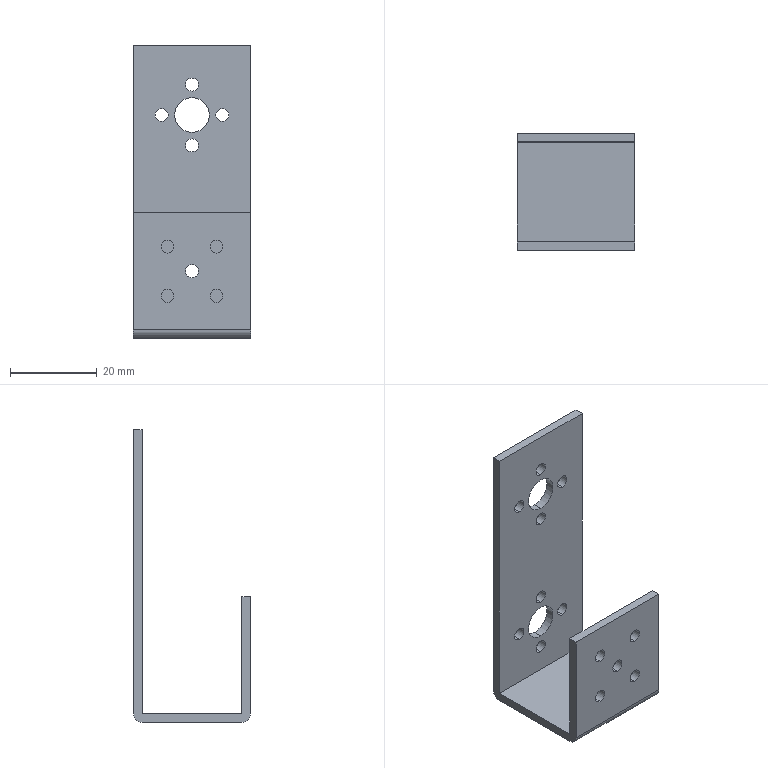Part | SolidWorks | features ICE 5, Extrusion 1, Fillet 1 | 1 solid | 42 faces | box 27 x 27 x 67.5 mm | volume 6022 mm3 | cylinder 32 | plane 10 | commonest cylinder face diameters 3 x26 8 x4 4 x2
STEP:
#1=CARTESIAN_POINT('',(0.,11.5,46.));
#2=VERTEX_POINT('',#1);
#3=CARTESIAN_POINT('',(0.,11.5,43.));
#4=VERTEX_POINT('',#3);
#5=CARTESIAN_POINT('',(0.,11.5,44.5));
#6=DIRECTION('',(0.,-1.,0.));
#7=DIRECTION('',(-1.,0.,0.));
#8=AXIS2_PLACEMENT_3D('',#5,#6,#7);
#9=CIRCLE('',#8,1.5);
#10=EDGE_CURVE('',#2,#4,#9,.T.);
#11=ORIENTED_EDGE('',*,*,#10,.T.);
#12=CARTESIAN_POINT('',(0.,13.5,43.));
#13=VERTEX_POINT('',#12);
#14=CARTESIAN_POINT('',(0.,0.1863,43.));
#15=DIRECTION('',(0.,1.,0.));
#16=VECTOR('',#15,1000.);
#17=LINE('',#14,#16);
#18=EDGE_CURVE('',#4,#13,#17,.T.);
#19=ORIENTED_EDGE('',*,*,#18,.T.);
#20=CARTESIAN_POINT('',(0.,13.5,46.));
#21=VERTEX_POINT('',#20);
#22=CARTESIAN_POINT('',(0.,13.5,44.5));
#23=DIRECTION('',(0.,1.,0.));
#24=DIRECTION('',(0.,0.,1.));
#25=AXIS2_PLACEMENT_3D('',#22,#23,#24);
#26=CIRCLE('',#25,1.5);
#27=EDGE_CURVE('',#13,#21,#26,.T.);
#28=ORIENTED_EDGE('',*,*,#27,.T.);
#29=CARTESIAN_POINT('',(0.,0.1863,46.));
#30=DIRECTION('',(0.,1.,0.));
#31=VECTOR('',#30,1000.);
#32=LINE('',#29,#31);
#33=EDGE_CURVE('',#2,#21,#32,.T.);
#34=ORIENTED_EDGE('',*,*,#33,.F.);
#35=EDGE_LOOP('',(#11,#19,#28,#34));
#36=FACE_OUTER_BOUND('',#35,.T.);
#37=CARTESIAN_POINT('',(0.,0.1863,44.5));
#38=DIRECTION('',(0.,1.,0.));
#39=DIRECTION('',(0.,0.,1.));
#40=AXIS2_PLACEMENT_3D('',#37,#38,#39);
#41=CYLINDRICAL_SURFACE('',#40,1.5);
#42=ADVANCED_FACE('',(#36),#41,.F.);
#43=CARTESIAN_POINT('',(7.,11.5,53.));
#44=VERTEX_POINT('',#43);
#45=CARTESIAN_POINT('',(7.,11.5,50.));
#46=VERTEX_POINT('',#45);
#47=CARTESIAN_POINT('',(7.,11.5,51.5));
#48=DIRECTION('',(0.,-1.,0.));
#49=DIRECTION('',(-1.,0.,0.));
#50=AXIS2_PLACEMENT_3D('',#47,#48,#49);
#51=CIRCLE('',#50,1.5);
#52=EDGE_CURVE('',#44,#46,#51,.T.);
#53=ORIENTED_EDGE('',*,*,#52,.T.);
#54=CARTESIAN_POINT('',(7.,13.5,50.));
#55=VERTEX_POINT('',#54);
#56=CARTESIAN_POINT('',(7.,0.1863,50.));
#57=DIRECTION('',(0.,1.,0.));
#58=VECTOR('',#57,1000.);
#59=LINE('',#56,#58);
#60=EDGE_CURVE('',#46,#55,#59,.T.);
#61=ORIENTED_EDGE('',*,*,#60,.T.);
#62=CARTESIAN_POINT('',(7.,13.5,53.));
#63=VERTEX_POINT('',#62);
#64=CARTESIAN_POINT('',(7.,13.5,51.5));
#65=DIRECTION('',(0.,1.,0.));
#66=DIRECTION('',(0.,0.,1.));
#67=AXIS2_PLACEMENT_3D('',#64,#65,#66);
#68=CIRCLE('',#67,1.5);
#69=EDGE_CURVE('',#55,#63,#68,.T.);
#70=ORIENTED_EDGE('',*,*,#69,.T.);
#71=CARTESIAN_POINT('',(7.,0.1863,53.));
#72=DIRECTION('',(0.,1.,0.));
#73=VECTOR('',#72,1000.);
#74=LINE('',#71,#73);
#75=EDGE_CURVE('',#44,#63,#74,.T.);
#76=ORIENTED_EDGE('',*,*,#75,.F.);
#77=EDGE_LOOP('',(#53,#61,#70,#76));
#78=FACE_OUTER_BOUND('',#77,.T.);
#79=CARTESIAN_POINT('',(7.,0.1863,51.5));
#80=DIRECTION('',(0.,1.,0.));
#81=DIRECTION('',(0.,0.,1.));
#82=AXIS2_PLACEMENT_3D('',#79,#80,#81);
#83=CYLINDRICAL_SURFACE('',#82,1.5);
#84=ADVANCED_FACE('',(#78),#83,.F.);
#85=CARTESIAN_POINT('',(0.,11.5,60.));
#86=VERTEX_POINT('',#85);
#87=CARTESIAN_POINT('',(0.,11.5,57.));
#88=VERTEX_POINT('',#87);
#89=CARTESIAN_POINT('',(0.,11.5,58.5));
#90=DIRECTION('',(0.,-1.,0.));
#91=DIRECTION('',(-1.,0.,0.));
#92=AXIS2_PLACEMENT_3D('',#89,#90,#91);
#93=CIRCLE('',#92,1.5);
#94=EDGE_CURVE('',#86,#88,#93,.T.);
#95=ORIENTED_EDGE('',*,*,#94,.T.);
#96=CARTESIAN_POINT('',(0.,13.5,57.));
#97=VERTEX_POINT('',#96);
#98=CARTESIAN_POINT('',(0.,0.1863,57.));
#99=DIRECTION('',(0.,1.,0.));
#100=VECTOR('',#99,1000.);
#101=LINE('',#98,#100);
#102=EDGE_CURVE('',#88,#97,#101,.T.);
#103=ORIENTED_EDGE('',*,*,#102,.T.);
#104=CARTESIAN_POINT('',(0.,13.5,60.));
#105=VERTEX_POINT('',#104);
#106=CARTESIAN_POINT('',(0.,13.5,58.5));
#107=DIRECTION('',(0.,1.,0.));
#108=DIRECTION('',(0.,0.,1.));
#109=AXIS2_PLACEMENT_3D('',#106,#107,#108);
#110=CIRCLE('',#109,1.5);
#111=EDGE_CURVE('',#97,#105,#110,.T.);
#112=ORIENTED_EDGE('',*,*,#111,.T.);
#113=CARTESIAN_POINT('',(0.,0.1863,60.));
#114=DIRECTION('',(0.,1.,0.));
#115=VECTOR('',#114,1000.);
#116=LINE('',#113,#115);
#117=EDGE_CURVE('',#86,#105,#116,.T.);
#118=ORIENTED_EDGE('',*,*,#117,.F.);
#119=EDGE_LOOP('',(#95,#103,#112,#118));
#120=FACE_OUTER_BOUND('',#119,.T.);
#121=CARTESIAN_POINT('',(0.,0.1863,58.5));
#122=DIRECTION('',(0.,1.,0.));
#123=DIRECTION('',(0.,0.,1.));
#124=AXIS2_PLACEMENT_3D('',#121,#122,#123);
#125=CYLINDRICAL_SURFACE('',#124,1.5);
#126=ADVANCED_FACE('',(#120),#125,.F.);
#127=CARTESIAN_POINT('',(-7.,11.5,53.));
#128=VERTEX_POINT('',#127);
#129=CARTESIAN_POINT('',(-7.,11.5,50.));
#130=VERTEX_POINT('',#129);
#131=CARTESIAN_POINT('',(-7.,11.5,51.5));
#132=DIRECTION('',(0.,-1.,0.));
#133=DIRECTION('',(-1.,0.,0.));
#134=AXIS2_PLACEMENT_3D('',#131,#132,#133);
#135=CIRCLE('',#134,1.5);
#136=EDGE_CURVE('',#128,#130,#135,.T.);
#137=ORIENTED_EDGE('',*,*,#136,.T.);
#138=CARTESIAN_POINT('',(-7.,13.5,50.));
#139=VERTEX_POINT('',#138);
#140=CARTESIAN_POINT('',(-7.,0.1863,50.));
#141=DIRECTION('',(0.,1.,0.));
#142=VECTOR('',#141,1000.);
#143=LINE('',#140,#142);
#144=EDGE_CURVE('',#130,#139,#143,.T.);
#145=ORIENTED_EDGE('',*,*,#144,.T.);
#146=CARTESIAN_POINT('',(-7.,13.5,53.));
#147=VERTEX_POINT('',#146);
#148=CARTESIAN_POINT('',(-7.,13.5,51.5));
#149=DIRECTION('',(0.,1.,0.));
#150=DIRECTION('',(0.,0.,1.));
#151=AXIS2_PLACEMENT_3D('',#148,#149,#150);
#152=CIRCLE('',#151,1.5);
#153=EDGE_CURVE('',#139,#147,#152,.T.);
#154=ORIENTED_EDGE('',*,*,#153,.T.);
#155=CARTESIAN_POINT('',(-7.,0.1863,53.));
#156=DIRECTION('',(0.,1.,0.));
#157=VECTOR('',#156,1000.);
#158=LINE('',#155,#157);
#159=EDGE_CURVE('',#128,#147,#158,.T.);
#160=ORIENTED_EDGE('',*,*,#159,.F.);
#161=EDGE_LOOP('',(#137,#145,#154,#160));
#162=FACE_OUTER_BOUND('',#161,.T.);
#163=CARTESIAN_POINT('',(-7.,0.1863,51.5));
#164=DIRECTION('',(0.,1.,0.));
#165=DIRECTION('',(0.,0.,1.));
#166=AXIS2_PLACEMENT_3D('',#163,#164,#165);
#167=CYLINDRICAL_SURFACE('',#166,1.5);
#168=ADVANCED_FACE('',(#162),#167,.F.);
#169=CARTESIAN_POINT('',(0.,11.5,55.5));
#170=VERTEX_POINT('',#169);
#171=CARTESIAN_POINT('',(0.,11.5,47.5));
#172=VERTEX_POINT('',#171);
#173=CARTESIAN_POINT('',(0.,11.5,51.5));
#174=DIRECTION('',(0.,-1.,0.));
#175=DIRECTION('',(-1.,0.,0.));
#176=AXIS2_PLACEMENT_3D('',#173,#174,#175);
#177=CIRCLE('',#176,4.);
#178=EDGE_CURVE('',#170,#172,#177,.T.);
#179=ORIENTED_EDGE('',*,*,#178,.T.);
#180=CARTESIAN_POINT('',(0.,13.5,47.5));
#181=VERTEX_POINT('',#180);
#182=CARTESIAN_POINT('',(0.,0.1863,47.5));
#183=DIRECTION('',(0.,1.,0.));
#184=VECTOR('',#183,1000.);
#185=LINE('',#182,#184);
#186=EDGE_CURVE('',#172,#181,#185,.T.);
#187=ORIENTED_EDGE('',*,*,#186,.T.);
#188=CARTESIAN_POINT('',(0.,13.5,55.5));
#189=VERTEX_POINT('',#188);
#190=CARTESIAN_POINT('',(0.,13.5,51.5));
#191=DIRECTION('',(0.,1.,0.));
#192=DIRECTION('',(0.,0.,1.));
#193=AXIS2_PLACEMENT_3D('',#190,#191,#192);
#194=CIRCLE('',#193,4.);
#195=EDGE_CURVE('',#181,#189,#194,.T.);
#196=ORIENTED_EDGE('',*,*,#195,.T.);
#197=CARTESIAN_POINT('',(0.,0.1863,55.5));
#198=DIRECTION('',(0.,1.,0.));
#199=VECTOR('',#198,1000.);
#200=LINE('',#197,#199);
#201=EDGE_CURVE('',#170,#189,#200,.T.);
#202=ORIENTED_EDGE('',*,*,#201,.F.);
#203=EDGE_LOOP('',(#179,#187,#196,#202));
#204=FACE_OUTER_BOUND('',#203,.T.);
#205=CARTESIAN_POINT('',(0.,0.1863,51.5));
#206=DIRECTION('',(0.,1.,0.));
#207=DIRECTION('',(0.,0.,1.));
#208=AXIS2_PLACEMENT_3D('',#205,#206,#207);
#209=CYLINDRICAL_SURFACE('',#208,4.);
#210=ADVANCED_FACE('',(#204),#209,.F.);
#211=CARTESIAN_POINT('',(-5.657,-11.5,8.343));
#212=VERTEX_POINT('',#211);
#213=CARTESIAN_POINT('',(-5.657,-11.5,11.343));
#214=VERTEX_POINT('',#213);
#215=CARTESIAN_POINT('',(-5.657,-11.5,9.843));
#216=DIRECTION('',(0.,1.,0.));
#217=DIRECTION('',(1.,0.,0.));
#218=AXIS2_PLACEMENT_3D('',#215,#216,#217);
#219=CIRCLE('',#218,1.5);
#220=EDGE_CURVE('',#212,#214,#219,.T.);
#221=ORIENTED_EDGE('',*,*,#220,.T.);
#222=CARTESIAN_POINT('',(-5.657,-13.5,11.343));
#223=VERTEX_POINT('',#222);
#224=CARTESIAN_POINT('',(-5.657,13.501,11.343));
#225=DIRECTION('',(0.,-1.,0.));
#226=VECTOR('',#225,1000.);
#227=LINE('',#224,#226);
#228=EDGE_CURVE('',#214,#223,#227,.T.);
#229=ORIENTED_EDGE('',*,*,#228,.T.);
#230=CARTESIAN_POINT('',(-5.657,-13.5,8.343));
#231=VERTEX_POINT('',#230);
#232=CARTESIAN_POINT('',(-5.657,-13.5,9.843));
#233=DIRECTION('',(0.,-1.,0.));
#234=DIRECTION('',(0.,0.,-1.));
#235=AXIS2_PLACEMENT_3D('',#232,#233,#234);
#236=CIRCLE('',#235,1.5);
#237=EDGE_CURVE('',#223,#231,#236,.T.);
#238=ORIENTED_EDGE('',*,*,#237,.T.);
#239=CARTESIAN_POINT('',(-5.657,13.501,8.343));
#240=DIRECTION('',(0.,-1.,0.));
#241=VECTOR('',#240,1000.);
#242=LINE('',#239,#241);
#243=EDGE_CURVE('',#212,#231,#242,.T.);
#244=ORIENTED_EDGE('',*,*,#243,.F.);
#245=EDGE_LOOP('',(#221,#229,#238,#244));
#246=FACE_OUTER_BOUND('',#245,.T.);
#247=CARTESIAN_POINT('',(-5.657,13.501,9.843));
#248=DIRECTION('',(0.,-1.,0.));
#249=DIRECTION('',(0.,0.,-1.));
#250=AXIS2_PLACEMENT_3D('',#247,#248,#249);
#251=CYLINDRICAL_SURFACE('',#250,1.5);
#252=ADVANCED_FACE('',(#246),#251,.F.);
#253=CARTESIAN_POINT('',(5.657,-11.5,8.343));
#254=VERTEX_POINT('',#253);
#255=CARTESIAN_POINT('',(5.657,-11.5,11.343));
#256=VERTEX_POINT('',#255);
#257=CARTESIAN_POINT('',(5.657,-11.5,9.843));
#258=DIRECTION('',(0.,1.,0.));
#259=DIRECTION('',(1.,0.,0.));
#260=AXIS2_PLACEMENT_3D('',#257,#258,#259);
#261=CIRCLE('',#260,1.5);
#262=EDGE_CURVE('',#254,#256,#261,.T.);
#263=ORIENTED_EDGE('',*,*,#262,.T.);
#264=CARTESIAN_POINT('',(5.657,-13.5,11.343));
#265=VERTEX_POINT('',#264);
#266=CARTESIAN_POINT('',(5.657,13.501,11.343));
#267=DIRECTION('',(0.,-1.,0.));
#268=VECTOR('',#267,1000.);
#269=LINE('',#266,#268);
#270=EDGE_CURVE('',#256,#265,#269,.T.);
#271=ORIENTED_EDGE('',*,*,#270,.T.);
#272=CARTESIAN_POINT('',(5.657,-13.5,8.343));
#273=VERTEX_POINT('',#272);
#274=CARTESIAN_POINT('',(5.657,-13.5,9.843));
#275=DIRECTION('',(0.,-1.,0.));
#276=DIRECTION('',(0.,0.,-1.));
#277=AXIS2_PLACEMENT_3D('',#274,#275,#276);
#278=CIRCLE('',#277,1.5);
#279=EDGE_CURVE('',#265,#273,#278,.T.);
#280=ORIENTED_EDGE('',*,*,#279,.T.);
#281=CARTESIAN_POINT('',(5.657,13.501,8.343));
#282=DIRECTION('',(0.,-1.,0.));
#283=VECTOR('',#282,1000.);
#284=LINE('',#281,#283);
#285=EDGE_CURVE('',#254,#273,#284,.T.);
#286=ORIENTED_EDGE('',*,*,#285,.F.);
#287=EDGE_LOOP('',(#263,#271,#280,#286));
#288=FACE_OUTER_BOUND('',#287,.T.);
#289=CARTESIAN_POINT('',(5.657,13.501,9.843));
#290=DIRECTION('',(0.,-1.,0.));
#291=DIRECTION('',(0.,0.,-1.));
#292=AXIS2_PLACEMENT_3D('',#289,#290,#291);
#293=CYLINDRICAL_SURFACE('',#292,1.5);
#294=ADVANCED_FACE('',(#288),#293,.F.);
#295=CARTESIAN_POINT('',(5.657,-11.5,19.657));
#296=VERTEX_POINT('',#295);
#297=CARTESIAN_POINT('',(5.657,-11.5,22.657));
#298=VERTEX_POINT('',#297);
#299=CARTESIAN_POINT('',(5.657,-11.5,21.157));
#300=DIRECTION('',(0.,1.,0.));
#301=DIRECTION('',(1.,0.,0.));
#302=AXIS2_PLACEMENT_3D('',#299,#300,#301);
#303=CIRCLE('',#302,1.5);
#304=EDGE_CURVE('',#296,#298,#303,.T.);
#305=ORIENTED_EDGE('',*,*,#304,.T.);
#306=CARTESIAN_POINT('',(5.657,-13.5,22.657));
#307=VERTEX_POINT('',#306);
#308=CARTESIAN_POINT('',(5.657,13.501,22.657));
#309=DIRECTION('',(0.,-1.,0.));
#310=VECTOR('',#309,1000.);
#311=LINE('',#308,#310);
#312=EDGE_CURVE('',#298,#307,#311,.T.);
#313=ORIENTED_EDGE('',*,*,#312,.T.);
#314=CARTESIAN_POINT('',(5.657,-13.5,19.657));
#315=VERTEX_POINT('',#314);
#316=CARTESIAN_POINT('',(5.657,-13.5,21.157));
#317=DIRECTION('',(0.,-1.,0.));
#318=DIRECTION('',(0.,0.,-1.));
#319=AXIS2_PLACEMENT_3D('',#316,#317,#318);
#320=CIRCLE('',#319,1.5);
#321=EDGE_CURVE('',#307,#315,#320,.T.);
#322=ORIENTED_EDGE('',*,*,#321,.T.);
#323=CARTESIAN_POINT('',(5.657,13.501,19.657));
#324=DIRECTION('',(0.,-1.,0.));
#325=VECTOR('',#324,1000.);
#326=LINE('',#323,#325);
#327=EDGE_CURVE('',#296,#315,#326,.T.);
#328=ORIENTED_EDGE('',*,*,#327,.F.);
#329=EDGE_LOOP('',(#305,#313,#322,#328));
#330=FACE_OUTER_BOUND('',#329,.T.);
#331=CARTESIAN_POINT('',(5.657,13.501,21.157));
#332=DIRECTION('',(0.,-1.,0.));
#333=DIRECTION('',(0.,0.,-1.));
#334=AXIS2_PLACEMENT_3D('',#331,#332,#333);
#335=CYLINDRICAL_SURFACE('',#334,1.5);
#336=ADVANCED_FACE('',(#330),#335,.F.);
#337=CARTESIAN_POINT('',(-5.657,-11.5,19.657));
#338=VERTEX_POINT('',#337);
#339=CARTESIAN_POINT('',(-5.657,-11.5,22.657));
#340=VERTEX_POINT('',#339);
#341=CARTESIAN_POINT('',(-5.657,-11.5,21.157));
#342=DIRECTION('',(0.,1.,0.));
#343=DIRECTION('',(1.,0.,0.));
#344=AXIS2_PLACEMENT_3D('',#341,#342,#343);
#345=CIRCLE('',#344,1.5);
#346=EDGE_CURVE('',#338,#340,#345,.T.);
#347=ORIENTED_EDGE('',*,*,#346,.T.);
#348=CARTESIAN_POINT('',(-5.657,-13.5,22.657));
#349=VERTEX_POINT('',#348);
#350=CARTESIAN_POINT('',(-5.657,13.501,22.657));
#351=DIRECTION('',(0.,-1.,0.));
#352=VECTOR('',#351,1000.);
#353=LINE('',#350,#352);
#354=EDGE_CURVE('',#340,#349,#353,.T.);
#355=ORIENTED_EDGE('',*,*,#354,.T.);
#356=CARTESIAN_POINT('',(-5.657,-13.5,19.657));
#357=VERTEX_POINT('',#356);
#358=CARTESIAN_POINT('',(-5.657,-13.5,21.157));
#359=DIRECTION('',(0.,-1.,0.));
#360=DIRECTION('',(0.,0.,-1.));
#361=AXIS2_PLACEMENT_3D('',#358,#359,#360);
#362=CIRCLE('',#361,1.5);
#363=EDGE_CURVE('',#349,#357,#362,.T.);
#364=ORIENTED_EDGE('',*,*,#363,.T.);
#365=CARTESIAN_POINT('',(-5.657,13.501,19.657));
#366=DIRECTION('',(0.,-1.,0.));
#367=VECTOR('',#366,1000.);
#368=LINE('',#365,#367);
#369=EDGE_CURVE('',#338,#357,#368,.T.);
#370=ORIENTED_EDGE('',*,*,#369,.F.);
#371=EDGE_LOOP('',(#347,#355,#364,#370));
#372=FACE_OUTER_BOUND('',#371,.T.);
#373=CARTESIAN_POINT('',(-5.657,13.501,21.157));
#374=DIRECTION('',(0.,-1.,0.));
#375=DIRECTION('',(0.,0.,-1.));
#376=AXIS2_PLACEMENT_3D('',#373,#374,#375);
#377=CYLINDRICAL_SURFACE('',#376,1.5);
#378=ADVANCED_FACE('',(#372),#377,.F.);
#379=CARTESIAN_POINT('',(0.,-11.5,14.));
#380=VERTEX_POINT('',#379);
#381=CARTESIAN_POINT('',(0.,-11.5,17.));
#382=VERTEX_POINT('',#381);
#383=CARTESIAN_POINT('',(0.,-11.5,15.5));
#384=DIRECTION('',(0.,1.,0.));
#385=DIRECTION('',(1.,0.,0.));
#386=AXIS2_PLACEMENT_3D('',#383,#384,#385);
#387=CIRCLE('',#386,1.5);
#388=EDGE_CURVE('',#380,#382,#387,.T.);
#389=ORIENTED_EDGE('',*,*,#388,.T.);
#390=CARTESIAN_POINT('',(0.,-13.5,17.));
#391=VERTEX_POINT('',#390);
#392=CARTESIAN_POINT('',(0.,13.501,17.));
#393=DIRECTION('',(0.,-1.,0.));
#394=VECTOR('',#393,1000.);
#395=LINE('',#392,#394);
#396=EDGE_CURVE('',#382,#391,#395,.T.);
#397=ORIENTED_EDGE('',*,*,#396,.T.);
#398=CARTESIAN_POINT('',(0.,-13.5,14.));
#399=VERTEX_POINT('',#398);
#400=CARTESIAN_POINT('',(0.,-13.5,15.5));
#401=DIRECTION('',(0.,-1.,0.));
#402=DIRECTION('',(0.,0.,-1.));
#403=AXIS2_PLACEMENT_3D('',#400,#401,#402);
#404=CIRCLE('',#403,1.5);
#405=EDGE_CURVE('',#391,#399,#404,.T.);
#406=ORIENTED_EDGE('',*,*,#405,.T.);
#407=CARTESIAN_POINT('',(0.,13.501,14.));
#408=DIRECTION('',(0.,-1.,0.));
#409=VECTOR('',#408,1000.);
#410=LINE('',#407,#409);
#411=EDGE_CURVE('',#380,#399,#410,.T.);
#412=ORIENTED_EDGE('',*,*,#411,.F.);
#413=EDGE_LOOP('',(#389,#397,#406,#412));
#414=FACE_OUTER_BOUND('',#413,.T.);
#415=CARTESIAN_POINT('',(0.,13.501,15.5));
#416=DIRECTION('',(0.,-1.,0.));
#417=DIRECTION('',(0.,0.,-1.));
#418=AXIS2_PLACEMENT_3D('',#415,#416,#417);
#419=CYLINDRICAL_SURFACE('',#418,1.5);
#420=ADVANCED_FACE('',(#414),#419,.F.);
#421=CARTESIAN_POINT('',(0.,11.5,10.));
#422=VERTEX_POINT('',#421);
#423=CARTESIAN_POINT('',(0.,11.5,7.));
#424=VERTEX_POINT('',#423);
#425=CARTESIAN_POINT('',(0.,11.5,8.5));
#426=DIRECTION('',(0.,-1.,0.));
#427=DIRECTION('',(-1.,0.,0.));
#428=AXIS2_PLACEMENT_3D('',#425,#426,#427);
#429=CIRCLE('',#428,1.5);
#430=EDGE_CURVE('',#422,#424,#429,.T.);
#431=ORIENTED_EDGE('',*,*,#430,.T.);
#432=CARTESIAN_POINT('',(0.,13.5,7.));
#433=VERTEX_POINT('',#432);
#434=CARTESIAN_POINT('',(0.,-13.501,7.));
#435=DIRECTION('',(0.,1.,0.));
#436=VECTOR('',#435,1000.);
#437=LINE('',#434,#436);
#438=EDGE_CURVE('',#424,#433,#437,.T.);
#439=ORIENTED_EDGE('',*,*,#438,.T.);
#440=CARTESIAN_POINT('',(0.,13.5,10.));
#441=VERTEX_POINT('',#440);
#442=CARTESIAN_POINT('',(0.,13.5,8.5));
#443=DIRECTION('',(0.,1.,0.));
#444=DIRECTION('',(0.,0.,1.));
#445=AXIS2_PLACEMENT_3D('',#442,#443,#444);
#446=CIRCLE('',#445,1.5);
#447=EDGE_CURVE('',#433,#441,#446,.T.);
#448=ORIENTED_EDGE('',*,*,#447,.T.);
#449=CARTESIAN_POINT('',(0.,-13.501,10.));
#450=DIRECTION('',(0.,1.,0.));
#451=VECTOR('',#450,1000.);
#452=LINE('',#449,#451);
#453=EDGE_CURVE('',#422,#441,#452,.T.);
#454=ORIENTED_EDGE('',*,*,#453,.F.);
#455=EDGE_LOOP('',(#431,#439,#448,#454));
#456=FACE_OUTER_BOUND('',#455,.T.);
#457=CARTESIAN_POINT('',(0.,-13.501,8.5));
#458=DIRECTION('',(0.,1.,0.));
#459=DIRECTION('',(0.,0.,1.));
#460=AXIS2_PLACEMENT_3D('',#457,#458,#459);
#461=CYLINDRICAL_SURFACE('',#460,1.5);
#462=ADVANCED_FACE('',(#456),#461,.F.);
#463=CARTESIAN_POINT('',(7.,11.5,17.));
#464=VERTEX_POINT('',#463);
#465=CARTESIAN_POINT('',(7.,11.5,14.));
#466=VERTEX_POINT('',#465);
#467=CARTESIAN_POINT('',(7.,11.5,15.5));
#468=DIRECTION('',(0.,-1.,0.));
#469=DIRECTION('',(-1.,0.,0.));
#470=AXIS2_PLACEMENT_3D('',#467,#468,#469);
#471=CIRCLE('',#470,1.5);
#472=EDGE_CURVE('',#464,#466,#471,.T.);
#473=ORIENTED_EDGE('',*,*,#472,.T.);
#474=CARTESIAN_POINT('',(7.,13.5,14.));
#475=VERTEX_POINT('',#474);
#476=CARTESIAN_POINT('',(7.,-13.501,14.));
#477=DIRECTION('',(0.,1.,0.));
#478=VECTOR('',#477,1000.);
#479=LINE('',#476,#478);
#480=EDGE_CURVE('',#466,#475,#479,.T.);
#481=ORIENTED_EDGE('',*,*,#480,.T.);
#482=CARTESIAN_POINT('',(7.,13.5,17.));
#483=VERTEX_POINT('',#482);
#484=CARTESIAN_POINT('',(7.,13.5,15.5));
#485=DIRECTION('',(0.,1.,0.));
#486=DIRECTION('',(0.,0.,1.));
#487=AXIS2_PLACEMENT_3D('',#484,#485,#486);
#488=CIRCLE('',#487,1.5);
#489=EDGE_CURVE('',#475,#483,#488,.T.);
#490=ORIENTED_EDGE('',*,*,#489,.T.);
#491=CARTESIAN_POINT('',(7.,-13.501,17.));
#492=DIRECTION('',(0.,1.,0.));
#493=VECTOR('',#492,1000.);
#494=LINE('',#491,#493);
#495=EDGE_CURVE('',#464,#483,#494,.T.);
#496=ORIENTED_EDGE('',*,*,#495,.F.);
#497=EDGE_LOOP('',(#473,#481,#490,#496));
#498=FACE_OUTER_BOUND('',#497,.T.);
#499=CARTESIAN_POINT('',(7.,-13.501,15.5));
#500=DIRECTION('',(0.,1.,0.));
#501=DIRECTION('',(0.,0.,1.));
#502=AXIS2_PLACEMENT_3D('',#499,#500,#501);
#503=CYLINDRICAL_SURFACE('',#502,1.5);
#504=ADVANCED_FACE('',(#498),#503,.F.);
#505=CARTESIAN_POINT('',(0.,11.5,24.));
#506=VERTEX_POINT('',#505);
#507=CARTESIAN_POINT('',(0.,11.5,21.));
#508=VERTEX_POINT('',#507);
#509=CARTESIAN_POINT('',(0.,11.5,22.5));
#510=DIRECTION('',(0.,-1.,0.));
#511=DIRECTION('',(-1.,0.,0.));
#512=AXIS2_PLACEMENT_3D('',#509,#510,#511);
#513=CIRCLE('',#512,1.5);
#514=EDGE_CURVE('',#506,#508,#513,.T.);
#515=ORIENTED_EDGE('',*,*,#514,.T.);
#516=CARTESIAN_POINT('',(0.,13.5,21.));
#517=VERTEX_POINT('',#516);
#518=CARTESIAN_POINT('',(0.,-13.501,21.));
#519=DIRECTION('',(0.,1.,0.));
#520=VECTOR('',#519,1000.);
#521=LINE('',#518,#520);
#522=EDGE_CURVE('',#508,#517,#521,.T.);
#523=ORIENTED_EDGE('',*,*,#522,.T.);
#524=CARTESIAN_POINT('',(0.,13.5,24.));
#525=VERTEX_POINT('',#524);
#526=CARTESIAN_POINT('',(0.,13.5,22.5));
#527=DIRECTION('',(0.,1.,0.));
#528=DIRECTION('',(0.,0.,1.));
#529=AXIS2_PLACEMENT_3D('',#526,#527,#528);
#530=CIRCLE('',#529,1.5);
#531=EDGE_CURVE('',#517,#525,#530,.T.);
#532=ORIENTED_EDGE('',*,*,#531,.T.);
#533=CARTESIAN_POINT('',(0.,-13.501,24.));
#534=DIRECTION('',(0.,1.,0.));
#535=VECTOR('',#534,1000.);
#536=LINE('',#533,#535);
#537=EDGE_CURVE('',#506,#525,#536,.T.);
#538=ORIENTED_EDGE('',*,*,#537,.F.);
#539=EDGE_LOOP('',(#515,#523,#532,#538));
#540=FACE_OUTER_BOUND('',#539,.T.);
#541=CARTESIAN_POINT('',(0.,-13.501,22.5));
#542=DIRECTION('',(0.,1.,0.));
#543=DIRECTION('',(0.,0.,1.));
#544=AXIS2_PLACEMENT_3D('',#541,#542,#543);
#545=CYLINDRICAL_SURFACE('',#544,1.5);
#546=ADVANCED_FACE('',(#540),#545,.F.);
#547=CARTESIAN_POINT('',(-7.,11.5,17.));
#548=VERTEX_POINT('',#547);
#549=CARTESIAN_POINT('',(-7.,11.5,14.));
#550=VERTEX_POINT('',#549);
#551=CARTESIAN_POINT('',(-7.,11.5,15.5));
#552=DIRECTION('',(0.,-1.,0.));
#553=DIRECTION('',(-1.,0.,0.));
#554=AXIS2_PLACEMENT_3D('',#551,#552,#553);
#555=CIRCLE('',#554,1.5);
#556=EDGE_CURVE('',#548,#550,#555,.T.);
#557=ORIENTED_EDGE('',*,*,#556,.T.);
#558=CARTESIAN_POINT('',(-7.,13.5,14.));
#559=VERTEX_POINT('',#558);
#560=CARTESIAN_POINT('',(-7.,-13.501,14.));
#561=DIRECTION('',(0.,1.,0.));
#562=VECTOR('',#561,1000.);
#563=LINE('',#560,#562);
#564=EDGE_CURVE('',#550,#559,#563,.T.);
#565=ORIENTED_EDGE('',*,*,#564,.T.);
#566=CARTESIAN_POINT('',(-7.,13.5,17.));
#567=VERTEX_POINT('',#566);
#568=CARTESIAN_POINT('',(-7.,13.5,15.5));
#569=DIRECTION('',(0.,1.,0.));
#570=DIRECTION('',(0.,0.,1.));
#571=AXIS2_PLACEMENT_3D('',#568,#569,#570);
#572=CIRCLE('',#571,1.5);
#573=EDGE_CURVE('',#559,#567,#572,.T.);
#574=ORIENTED_EDGE('',*,*,#573,.T.);
#575=CARTESIAN_POINT('',(-7.,-13.501,17.));
#576=DIRECTION('',(0.,1.,0.));
#577=VECTOR('',#576,1000.);
#578=LINE('',#575,#577);
#579=EDGE_CURVE('',#548,#567,#578,.T.);
#580=ORIENTED_EDGE('',*,*,#579,.F.);
#581=EDGE_LOOP('',(#557,#565,#574,#580));
#582=FACE_OUTER_BOUND('',#581,.T.);
#583=CARTESIAN_POINT('',(-7.,-13.501,15.5));
#584=DIRECTION('',(0.,1.,0.));
#585=DIRECTION('',(0.,0.,1.));
#586=AXIS2_PLACEMENT_3D('',#583,#584,#585);
#587=CYLINDRICAL_SURFACE('',#586,1.5);
#588=ADVANCED_FACE('',(#582),#587,.F.);
#589=CARTESIAN_POINT('',(0.,11.5,19.5));
#590=VERTEX_POINT('',#589);
#591=CARTESIAN_POINT('',(0.,11.5,11.5));
#592=VERTEX_POINT('',#591);
#593=CARTESIAN_POINT('',(0.,11.5,15.5));
#594=DIRECTION('',(0.,-1.,0.));
#595=DIRECTION('',(-1.,0.,0.));
#596=AXIS2_PLACEMENT_3D('',#593,#594,#595);
#597=CIRCLE('',#596,4.);
#598=EDGE_CURVE('',#590,#592,#597,.T.);
#599=ORIENTED_EDGE('',*,*,#598,.T.);
#600=CARTESIAN_POINT('',(0.,13.5,11.5));
#601=VERTEX_POINT('',#600);
#602=CARTESIAN_POINT('',(0.,-13.501,11.5));
#603=DIRECTION('',(0.,1.,0.));
#604=VECTOR('',#603,1000.);
#605=LINE('',#602,#604);
#606=EDGE_CURVE('',#592,#601,#605,.T.);
#607=ORIENTED_EDGE('',*,*,#606,.T.);
#608=CARTESIAN_POINT('',(0.,13.5,19.5));
#609=VERTEX_POINT('',#608);
#610=CARTESIAN_POINT('',(0.,13.5,15.5));
#611=DIRECTION('',(0.,1.,0.));
#612=DIRECTION('',(0.,0.,1.));
#613=AXIS2_PLACEMENT_3D('',#610,#611,#612);
#614=CIRCLE('',#613,4.);
#615=EDGE_CURVE('',#601,#609,#614,.T.);
#616=ORIENTED_EDGE('',*,*,#615,.T.);
#617=CARTESIAN_POINT('',(0.,-13.501,19.5));
#618=DIRECTION('',(0.,1.,0.));
#619=VECTOR('',#618,1000.);
#620=LINE('',#617,#619);
#621=EDGE_CURVE('',#590,#609,#620,.T.);
#622=ORIENTED_EDGE('',*,*,#621,.F.);
#623=EDGE_LOOP('',(#599,#607,#616,#622));
#624=FACE_OUTER_BOUND('',#623,.T.);
#625=CARTESIAN_POINT('',(0.,-13.501,15.5));
#626=DIRECTION('',(0.,1.,0.));
#627=DIRECTION('',(0.,0.,1.));
#628=AXIS2_PLACEMENT_3D('',#625,#626,#627);
#629=CYLINDRICAL_SURFACE('',#628,4.);
#630=ADVANCED_FACE('',(#624),#629,.F.);
#631=CARTESIAN_POINT('',(13.5,-11.5,0.));
#632=VERTEX_POINT('',#631);
#633=CARTESIAN_POINT('',(13.5,11.5,0.));
#634=VERTEX_POINT('',#633);
#635=CARTESIAN_POINT('',(13.5,13.5,0.));
#636=DIRECTION('',(0.,1.,0.));
#637=VECTOR('',#636,1000.);
#638=LINE('',#635,#637);
#639=EDGE_CURVE('',#632,#634,#638,.T.);
#640=ORIENTED_EDGE('',*,*,#639,.T.);
#641=CARTESIAN_POINT('',(13.5,13.5,2.));
#642=VERTEX_POINT('',#641);
#643=CARTESIAN_POINT('',(13.5,11.5,2.));
#644=DIRECTION('',(1.,0.,0.));
#645=DIRECTION('',(0.,-1.,0.));
#646=AXIS2_PLACEMENT_3D('',#643,#644,#645);
#647=CIRCLE('',#646,2.);
#648=EDGE_CURVE('',#634,#642,#647,.T.);
#649=ORIENTED_EDGE('',*,*,#648,.T.);
#650=CARTESIAN_POINT('',(13.5,13.5,67.5));
#651=VERTEX_POINT('',#650);
#652=CARTESIAN_POINT('',(13.5,13.5,29.));
#653=DIRECTION('',(0.,0.,-1.));
#654=VECTOR('',#653,1000.);
#655=LINE('',#652,#654);
#656=EDGE_CURVE('',#651,#642,#655,.T.);
#657=ORIENTED_EDGE('',*,*,#656,.F.);
#658=CARTESIAN_POINT('',(13.5,11.5,67.5));
#659=VERTEX_POINT('',#658);
#660=CARTESIAN_POINT('',(13.5,11.5,67.5));
#661=DIRECTION('',(0.,1.,0.));
#662=VECTOR('',#661,1000.);
#663=LINE('',#660,#662);
#664=EDGE_CURVE('',#659,#651,#663,.T.);
#665=ORIENTED_EDGE('',*,*,#664,.F.);
#666=CARTESIAN_POINT('',(13.5,11.5,2.));
#667=VERTEX_POINT('',#666);
#668=CARTESIAN_POINT('',(13.5,11.5,29.));
#669=DIRECTION('',(0.,0.,1.));
#670=VECTOR('',#669,1000.);
#671=LINE('',#668,#670);
#672=EDGE_CURVE('',#667,#659,#671,.T.);
#673=ORIENTED_EDGE('',*,*,#672,.F.);
#674=CARTESIAN_POINT('',(13.5,-11.5,2.));
#675=VERTEX_POINT('',#674);
#676=CARTESIAN_POINT('',(13.5,11.5,2.));
#677=DIRECTION('',(0.,1.,0.));
#678=VECTOR('',#677,1000.);
#679=LINE('',#676,#678);
#680=EDGE_CURVE('',#675,#667,#679,.T.);
#681=ORIENTED_EDGE('',*,*,#680,.F.);
#682=CARTESIAN_POINT('',(13.5,-11.5,29.));
#683=VERTEX_POINT('',#682);
#684=CARTESIAN_POINT('',(13.5,-11.5,29.));
#685=DIRECTION('',(0.,0.,-1.));
#686=VECTOR('',#685,1000.);
#687=LINE('',#684,#686);
#688=EDGE_CURVE('',#683,#675,#687,.T.);
#689=ORIENTED_EDGE('',*,*,#688,.F.);
#690=CARTESIAN_POINT('',(13.5,-13.5,29.));
#691=VERTEX_POINT('',#690);
#692=CARTESIAN_POINT('',(13.5,13.5,29.));
#693=DIRECTION('',(0.,1.,0.));
#694=VECTOR('',#693,1000.);
#695=LINE('',#692,#694);
#696=EDGE_CURVE('',#691,#683,#695,.T.);
#697=ORIENTED_EDGE('',*,*,#696,.F.);
#698=CARTESIAN_POINT('',(13.5,-13.5,2.));
#699=VERTEX_POINT('',#698);
#700=CARTESIAN_POINT('',(13.5,-13.5,29.));
#701=DIRECTION('',(0.,0.,-1.));
#702=VECTOR('',#701,1000.);
#703=LINE('',#700,#702);
#704=EDGE_CURVE('',#691,#699,#703,.T.);
#705=ORIENTED_EDGE('',*,*,#704,.T.);
#706=CARTESIAN_POINT('',(13.5,-11.5,2.));
#707=DIRECTION('',(1.,0.,0.));
#708=DIRECTION('',(0.,-1.,0.));
#709=AXIS2_PLACEMENT_3D('',#706,#707,#708);
#710=CIRCLE('',#709,2.);
#711=EDGE_CURVE('',#699,#632,#710,.T.);
#712=ORIENTED_EDGE('',*,*,#711,.T.);
#713=EDGE_LOOP('',(#640,#649,#657,#665,#673,#681,#689,#697,#705,#712));
#714=FACE_OUTER_BOUND('',#713,.T.);
#715=CARTESIAN_POINT('',(13.5,13.5,29.));
#716=DIRECTION('',(-1.,0.,0.));
#717=DIRECTION('',(0.,-1.,0.));
#718=AXIS2_PLACEMENT_3D('',#715,#716,#717);
#719=PLANE('',#718);
#720=ADVANCED_FACE('',(#714),#719,.F.);
#721=CARTESIAN_POINT('',(0.,13.5,44.5));
#722=DIRECTION('',(0.,1.,0.));
#723=DIRECTION('',(0.,0.,1.));
#724=AXIS2_PLACEMENT_3D('',#721,#722,#723);
#725=CIRCLE('',#724,1.5);
#726=EDGE_CURVE('',#21,#13,#725,.T.);
#727=ORIENTED_EDGE('',*,*,#726,.F.);
#728=ORIENTED_EDGE('',*,*,#27,.F.);
#729=EDGE_LOOP('',(#727,#728));
#730=FACE_BOUND('',#729,.T.);
#731=CARTESIAN_POINT('',(7.,13.5,51.5));
#732=DIRECTION('',(0.,1.,0.));
#733=DIRECTION('',(0.,0.,1.));
#734=AXIS2_PLACEMENT_3D('',#731,#732,#733);
#735=CIRCLE('',#734,1.5);
#736=EDGE_CURVE('',#63,#55,#735,.T.);
#737=ORIENTED_EDGE('',*,*,#736,.F.);
#738=ORIENTED_EDGE('',*,*,#69,.F.);
#739=EDGE_LOOP('',(#737,#738));
#740=FACE_BOUND('',#739,.T.);
#741=CARTESIAN_POINT('',(0.,13.5,58.5));
#742=DIRECTION('',(0.,1.,0.));
#743=DIRECTION('',(0.,0.,1.));
#744=AXIS2_PLACEMENT_3D('',#741,#742,#743);
#745=CIRCLE('',#744,1.5);
#746=EDGE_CURVE('',#105,#97,#745,.T.);
#747=ORIENTED_EDGE('',*,*,#746,.F.);
#748=ORIENTED_EDGE('',*,*,#111,.F.);
#749=EDGE_LOOP('',(#747,#748));
#750=FACE_BOUND('',#749,.T.);
#751=CARTESIAN_POINT('',(-7.,13.5,51.5));
#752=DIRECTION('',(0.,1.,0.));
#753=DIRECTION('',(0.,0.,1.));
#754=AXIS2_PLACEMENT_3D('',#751,#752,#753);
#755=CIRCLE('',#754,1.5);
#756=EDGE_CURVE('',#147,#139,#755,.T.);
#757=ORIENTED_EDGE('',*,*,#756,.F.);
#758=ORIENTED_EDGE('',*,*,#153,.F.);
#759=EDGE_LOOP('',(#757,#758));
#760=FACE_BOUND('',#759,.T.);
#761=CARTESIAN_POINT('',(0.,13.5,51.5));
#762=DIRECTION('',(0.,1.,0.));
#763=DIRECTION('',(0.,0.,1.));
#764=AXIS2_PLACEMENT_3D('',#761,#762,#763);
#765=CIRCLE('',#764,4.);
#766=EDGE_CURVE('',#189,#181,#765,.T.);
#767=ORIENTED_EDGE('',*,*,#766,.F.);
#768=ORIENTED_EDGE('',*,*,#195,.F.);
#769=EDGE_LOOP('',(#767,#768));
#770=FACE_BOUND('',#769,.T.);
#771=CARTESIAN_POINT('',(0.,13.5,8.5));
#772=DIRECTION('',(0.,1.,0.));
#773=DIRECTION('',(0.,0.,1.));
#774=AXIS2_PLACEMENT_3D('',#771,#772,#773);
#775=CIRCLE('',#774,1.5);
#776=EDGE_CURVE('',#441,#433,#775,.T.);
#777=ORIENTED_EDGE('',*,*,#776,.F.);
#778=ORIENTED_EDGE('',*,*,#447,.F.);
#779=EDGE_LOOP('',(#777,#778));
#780=FACE_BOUND('',#779,.T.);
#781=CARTESIAN_POINT('',(7.,13.5,15.5));
#782=DIRECTION('',(0.,1.,0.));
#783=DIRECTION('',(0.,0.,1.));
#784=AXIS2_PLACEMENT_3D('',#781,#782,#783);
#785=CIRCLE('',#784,1.5);
#786=EDGE_CURVE('',#483,#475,#785,.T.);
#787=ORIENTED_EDGE('',*,*,#786,.F.);
#788=ORIENTED_EDGE('',*,*,#489,.F.);
#789=EDGE_LOOP('',(#787,#788));
#790=FACE_BOUND('',#789,.T.);
#791=CARTESIAN_POINT('',(0.,13.5,22.5));
#792=DIRECTION('',(0.,1.,0.));
#793=DIRECTION('',(0.,0.,1.));
#794=AXIS2_PLACEMENT_3D('',#791,#792,#793);
#795=CIRCLE('',#794,1.5);
#796=EDGE_CURVE('',#525,#517,#795,.T.);
#797=ORIENTED_EDGE('',*,*,#796,.F.);
#798=ORIENTED_EDGE('',*,*,#531,.F.);
#799=EDGE_LOOP('',(#797,#798));
#800=FACE_BOUND('',#799,.T.);
#801=CARTESIAN_POINT('',(-7.,13.5,15.5));
#802=DIRECTION('',(0.,1.,0.));
#803=DIRECTION('',(0.,0.,1.));
#804=AXIS2_PLACEMENT_3D('',#801,#802,#803);
#805=CIRCLE('',#804,1.5);
#806=EDGE_CURVE('',#567,#559,#805,.T.);
#807=ORIENTED_EDGE('',*,*,#806,.F.);
#808=ORIENTED_EDGE('',*,*,#573,.F.);
#809=EDGE_LOOP('',(#807,#808));
#810=FACE_BOUND('',#809,.T.);
#811=CARTESIAN_POINT('',(0.,13.5,15.5));
#812=DIRECTION('',(0.,1.,0.));
#813=DIRECTION('',(0.,0.,1.));
#814=AXIS2_PLACEMENT_3D('',#811,#812,#813);
#815=CIRCLE('',#814,4.);
#816=EDGE_CURVE('',#609,#601,#815,.T.);
#817=ORIENTED_EDGE('',*,*,#816,.F.);
#818=ORIENTED_EDGE('',*,*,#615,.F.);
#819=EDGE_LOOP('',(#817,#818));
#820=FACE_BOUND('',#819,.T.);
#821=ORIENTED_EDGE('',*,*,#656,.T.);
#822=CARTESIAN_POINT('',(-13.5,13.5,2.));
#823=VERTEX_POINT('',#822);
#824=CARTESIAN_POINT('',(-13.5,13.5,2.));
#825=DIRECTION('',(-1.,0.,0.));
#826=VECTOR('',#825,1000.);
#827=LINE('',#824,#826);
#828=EDGE_CURVE('',#642,#823,#827,.T.);
#829=ORIENTED_EDGE('',*,*,#828,.T.);
#830=CARTESIAN_POINT('',(-13.5,13.5,67.5));
#831=VERTEX_POINT('',#830);
#832=CARTESIAN_POINT('',(-13.5,13.5,29.));
#833=DIRECTION('',(0.,0.,-1.));
#834=VECTOR('',#833,1000.);
#835=LINE('',#832,#834);
#836=EDGE_CURVE('',#831,#823,#835,.T.);
#837=ORIENTED_EDGE('',*,*,#836,.F.);
#838=CARTESIAN_POINT('',(13.5,13.5,67.5));
#839=DIRECTION('',(-1.,0.,0.));
#840=VECTOR('',#839,1000.);
#841=LINE('',#838,#840);
#842=EDGE_CURVE('',#651,#831,#841,.T.);
#843=ORIENTED_EDGE('',*,*,#842,.F.);
#844=EDGE_LOOP('',(#821,#829,#837,#843));
#845=FACE_OUTER_BOUND('',#844,.T.);
#846=CARTESIAN_POINT('',(-13.5,13.5,29.));
#847=DIRECTION('',(0.,-1.,0.));
#848=DIRECTION('',(0.,0.,-1.));
#849=AXIS2_PLACEMENT_3D('',#846,#847,#848);
#850=PLANE('',#849);
#851=ADVANCED_FACE('',(#730,#740,#750,#760,#770,#780,#790,#800,#810,#820,#845),#850,.F.);
#852=ORIENTED_EDGE('',*,*,#836,.T.);
#853=CARTESIAN_POINT('',(-13.5,11.5,0.));
#854=VERTEX_POINT('',#853);
#855=CARTESIAN_POINT('',(-13.5,11.5,2.));
#856=DIRECTION('',(-1.,0.,0.));
#857=DIRECTION('',(0.,1.,0.));
#858=AXIS2_PLACEMENT_3D('',#855,#856,#857);
#859=CIRCLE('',#858,2.);
#860=EDGE_CURVE('',#823,#854,#859,.T.);
#861=ORIENTED_EDGE('',*,*,#860,.T.);
#862=CARTESIAN_POINT('',(-13.5,-11.5,0.));
#863=VERTEX_POINT('',#862);
#864=CARTESIAN_POINT('',(-13.5,13.5,0.));
#865=DIRECTION('',(0.,-1.,0.));
#866=VECTOR('',#865,1000.);
#867=LINE('',#864,#866);
#868=EDGE_CURVE('',#854,#863,#867,.T.);
#869=ORIENTED_EDGE('',*,*,#868,.T.);
#870=CARTESIAN_POINT('',(-13.5,-13.5,2.));
#871=VERTEX_POINT('',#870);
#872=CARTESIAN_POINT('',(-13.5,-11.5,2.));
#873=DIRECTION('',(-1.,0.,0.));
#874=DIRECTION('',(0.,1.,0.));
#875=AXIS2_PLACEMENT_3D('',#872,#873,#874);
#876=CIRCLE('',#875,2.);
#877=EDGE_CURVE('',#863,#871,#876,.T.);
#878=ORIENTED_EDGE('',*,*,#877,.T.);
#879=CARTESIAN_POINT('',(-13.5,-13.5,29.));
#880=VERTEX_POINT('',#879);
#881=CARTESIAN_POINT('',(-13.5,-13.5,29.));
#882=DIRECTION('',(0.,0.,-1.));
#883=VECTOR('',#882,1000.);
#884=LINE('',#881,#883);
#885=EDGE_CURVE('',#880,#871,#884,.T.);
#886=ORIENTED_EDGE('',*,*,#885,.F.);
#887=CARTESIAN_POINT('',(-13.5,-11.5,29.));
#888=VERTEX_POINT('',#887);
#889=CARTESIAN_POINT('',(-13.5,13.5,29.));
#890=DIRECTION('',(0.,-1.,0.));
#891=VECTOR('',#890,1000.);
#892=LINE('',#889,#891);
#893=EDGE_CURVE('',#888,#880,#892,.T.);
#894=ORIENTED_EDGE('',*,*,#893,.F.);
#895=CARTESIAN_POINT('',(-13.5,-11.5,2.));
#896=VERTEX_POINT('',#895);
#897=CARTESIAN_POINT('',(-13.5,-11.5,29.));
#898=DIRECTION('',(0.,0.,-1.));
#899=VECTOR('',#898,1000.);
#900=LINE('',#897,#899);
#901=EDGE_CURVE('',#888,#896,#900,.T.);
#902=ORIENTED_EDGE('',*,*,#901,.T.);
#903=CARTESIAN_POINT('',(-13.5,11.5,2.));
#904=VERTEX_POINT('',#903);
#905=CARTESIAN_POINT('',(-13.5,11.5,2.));
#906=DIRECTION('',(0.,1.,0.));
#907=VECTOR('',#906,1000.);
#908=LINE('',#905,#907);
#909=EDGE_CURVE('',#896,#904,#908,.T.);
#910=ORIENTED_EDGE('',*,*,#909,.T.);
#911=CARTESIAN_POINT('',(-13.5,11.5,67.5));
#912=VERTEX_POINT('',#911);
#913=CARTESIAN_POINT('',(-13.5,11.5,29.));
#914=DIRECTION('',(0.,0.,1.));
#915=VECTOR('',#914,1000.);
#916=LINE('',#913,#915);
#917=EDGE_CURVE('',#904,#912,#916,.T.);
#918=ORIENTED_EDGE('',*,*,#917,.T.);
#919=CARTESIAN_POINT('',(-13.5,13.5,67.5));
#920=DIRECTION('',(0.,-1.,0.));
#921=VECTOR('',#920,1000.);
#922=LINE('',#919,#921);
#923=EDGE_CURVE('',#831,#912,#922,.T.);
#924=ORIENTED_EDGE('',*,*,#923,.F.);
#925=EDGE_LOOP('',(#852,#861,#869,#878,#886,#894,#902,#910,#918,#924));
#926=FACE_OUTER_BOUND('',#925,.T.);
#927=CARTESIAN_POINT('',(-13.5,13.5,29.));
#928=DIRECTION('',(1.,0.,0.));
#929=DIRECTION('',(0.,1.,0.));
#930=AXIS2_PLACEMENT_3D('',#927,#928,#929);
#931=PLANE('',#930);
#932=ADVANCED_FACE('',(#926),#931,.F.);
#933=CARTESIAN_POINT('',(-5.657,-13.5,9.843));
#934=DIRECTION('',(0.,-1.,0.));
#935=DIRECTION('',(0.,0.,-1.));
#936=AXIS2_PLACEMENT_3D('',#933,#934,#935);
#937=CIRCLE('',#936,1.5);
#938=EDGE_CURVE('',#231,#223,#937,.T.);
#939=ORIENTED_EDGE('',*,*,#938,.F.);
#940=ORIENTED_EDGE('',*,*,#237,.F.);
#941=EDGE_LOOP('',(#939,#940));
#942=FACE_BOUND('',#941,.T.);
#943=CARTESIAN_POINT('',(5.657,-13.5,9.843));
#944=DIRECTION('',(0.,-1.,0.));
#945=DIRECTION('',(0.,0.,-1.));
#946=AXIS2_PLACEMENT_3D('',#943,#944,#945);
#947=CIRCLE('',#946,1.5);
#948=EDGE_CURVE('',#273,#265,#947,.T.);
#949=ORIENTED_EDGE('',*,*,#948,.F.);
#950=ORIENTED_EDGE('',*,*,#279,.F.);
#951=EDGE_LOOP('',(#949,#950));
#952=FACE_BOUND('',#951,.T.);
#953=CARTESIAN_POINT('',(5.657,-13.5,21.157));
#954=DIRECTION('',(0.,-1.,0.));
#955=DIRECTION('',(0.,0.,-1.));
#956=AXIS2_PLACEMENT_3D('',#953,#954,#955);
#957=CIRCLE('',#956,1.5);
#958=EDGE_CURVE('',#315,#307,#957,.T.);
#959=ORIENTED_EDGE('',*,*,#958,.F.);
#960=ORIENTED_EDGE('',*,*,#321,.F.);
#961=EDGE_LOOP('',(#959,#960));
#962=FACE_BOUND('',#961,.T.);
#963=CARTESIAN_POINT('',(-5.657,-13.5,21.157));
#964=DIRECTION('',(0.,-1.,0.));
#965=DIRECTION('',(0.,0.,-1.));
#966=AXIS2_PLACEMENT_3D('',#963,#964,#965);
#967=CIRCLE('',#966,1.5);
#968=EDGE_CURVE('',#357,#349,#967,.T.);
#969=ORIENTED_EDGE('',*,*,#968,.F.);
#970=ORIENTED_EDGE('',*,*,#363,.F.);
#971=EDGE_LOOP('',(#969,#970));
#972=FACE_BOUND('',#971,.T.);
#973=CARTESIAN_POINT('',(0.,-13.5,15.5));
#974=DIRECTION('',(0.,-1.,0.));
#975=DIRECTION('',(0.,0.,-1.));
#976=AXIS2_PLACEMENT_3D('',#973,#974,#975);
#977=CIRCLE('',#976,1.5);
#978=EDGE_CURVE('',#399,#391,#977,.T.);
#979=ORIENTED_EDGE('',*,*,#978,.F.);
#980=ORIENTED_EDGE('',*,*,#405,.F.);
#981=EDGE_LOOP('',(#979,#980));
#982=FACE_BOUND('',#981,.T.);
#983=ORIENTED_EDGE('',*,*,#885,.T.);
#984=CARTESIAN_POINT('',(-13.5,-13.5,2.));
#985=DIRECTION('',(1.,0.,0.));
#986=VECTOR('',#985,1000.);
#987=LINE('',#984,#986);
#988=EDGE_CURVE('',#871,#699,#987,.T.);
#989=ORIENTED_EDGE('',*,*,#988,.T.);
#990=ORIENTED_EDGE('',*,*,#704,.F.);
#991=CARTESIAN_POINT('',(-13.5,-13.5,29.));
#992=DIRECTION('',(1.,0.,0.));
#993=VECTOR('',#992,1000.);
#994=LINE('',#991,#993);
#995=EDGE_CURVE('',#880,#691,#994,.T.);
#996=ORIENTED_EDGE('',*,*,#995,.F.);
#997=EDGE_LOOP('',(#983,#989,#990,#996));
#998=FACE_OUTER_BOUND('',#997,.T.);
#999=CARTESIAN_POINT('',(-13.5,-13.5,29.));
#1000=DIRECTION('',(0.,1.,0.));
#1001=DIRECTION('',(0.,0.,1.));
#1002=AXIS2_PLACEMENT_3D('',#999,#1000,#1001);
#1003=PLANE('',#1002);
#1004=ADVANCED_FACE('',(#942,#952,#962,#972,#982,#998),#1003,.F.);
#1005=CARTESIAN_POINT('',(-13.5,-11.5,29.));
#1006=DIRECTION('',(1.,0.,0.));
#1007=VECTOR('',#1006,1000.);
#1008=LINE('',#1005,#1007);
#1009=EDGE_CURVE('',#888,#683,#1008,.T.);
#1010=ORIENTED_EDGE('',*,*,#1009,.F.);
#1011=ORIENTED_EDGE('',*,*,#893,.T.);
#1012=ORIENTED_EDGE('',*,*,#995,.T.);
#1013=ORIENTED_EDGE('',*,*,#696,.T.);
#1014=EDGE_LOOP('',(#1010,#1011,#1012,#1013));
#1015=FACE_OUTER_BOUND('',#1014,.T.);
#1016=CARTESIAN_POINT('',(0.,0.,29.));
#1017=DIRECTION('',(0.,0.,1.));
#1018=DIRECTION('',(1.,0.,0.));
#1019=AXIS2_PLACEMENT_3D('',#1016,#1017,#1018);
#1020=PLANE('',#1019);
#1021=ADVANCED_FACE('',(#1015),#1020,.T.);
#1022=ORIENTED_EDGE('',*,*,#868,.F.);
#1023=CARTESIAN_POINT('',(0.,11.5,0.));
#1024=DIRECTION('',(1.,0.,0.));
#1025=VECTOR('',#1024,1000.);
#1026=LINE('',#1023,#1025);
#1027=EDGE_CURVE('',#854,#634,#1026,.T.);
#1028=ORIENTED_EDGE('',*,*,#1027,.T.);
#1029=ORIENTED_EDGE('',*,*,#639,.F.);
#1030=CARTESIAN_POINT('',(0.,-11.5,0.));
#1031=DIRECTION('',(-1.,0.,0.));
#1032=VECTOR('',#1031,1000.);
#1033=LINE('',#1030,#1032);
#1034=EDGE_CURVE('',#632,#863,#1033,.T.);
#1035=ORIENTED_EDGE('',*,*,#1034,.T.);
#1036=EDGE_LOOP('',(#1022,#1028,#1029,#1035));
#1037=FACE_OUTER_BOUND('',#1036,.T.);
#1038=CARTESIAN_POINT('',(0.,0.,0.));
#1039=DIRECTION('',(0.,0.,1.));
#1040=DIRECTION('',(1.,0.,0.));
#1041=AXIS2_PLACEMENT_3D('',#1038,#1039,#1040);
#1042=PLANE('',#1041);
#1043=ADVANCED_FACE('',(#1037),#1042,.F.);
#1044=ORIENTED_EDGE('',*,*,#10,.F.);
#1045=CARTESIAN_POINT('',(0.,11.5,44.5));
#1046=DIRECTION('',(0.,-1.,0.));
#1047=DIRECTION('',(-1.,0.,0.));
#1048=AXIS2_PLACEMENT_3D('',#1045,#1046,#1047);
#1049=CIRCLE('',#1048,1.5);
#1050=EDGE_CURVE('',#4,#2,#1049,.T.);
#1051=ORIENTED_EDGE('',*,*,#1050,.F.);
#1052=EDGE_LOOP('',(#1044,#1051));
#1053=FACE_BOUND('',#1052,.T.);
#1054=ORIENTED_EDGE('',*,*,#52,.F.);
#1055=CARTESIAN_POINT('',(7.,11.5,51.5));
#1056=DIRECTION('',(0.,-1.,0.));
#1057=DIRECTION('',(-1.,0.,0.));
#1058=AXIS2_PLACEMENT_3D('',#1055,#1056,#1057);
#1059=CIRCLE('',#1058,1.5);
#1060=EDGE_CURVE('',#46,#44,#1059,.T.);
#1061=ORIENTED_EDGE('',*,*,#1060,.F.);
#1062=EDGE_LOOP('',(#1054,#1061));
#1063=FACE_BOUND('',#1062,.T.);
#1064=ORIENTED_EDGE('',*,*,#94,.F.);
#1065=CARTESIAN_POINT('',(0.,11.5,58.5));
#1066=DIRECTION('',(0.,-1.,0.));
#1067=DIRECTION('',(-1.,0.,0.));
#1068=AXIS2_PLACEMENT_3D('',#1065,#1066,#1067);
#1069=CIRCLE('',#1068,1.5);
#1070=EDGE_CURVE('',#88,#86,#1069,.T.);
#1071=ORIENTED_EDGE('',*,*,#1070,.F.);
#1072=EDGE_LOOP('',(#1064,#1071));
#1073=FACE_BOUND('',#1072,.T.);
#1074=ORIENTED_EDGE('',*,*,#136,.F.);
#1075=CARTESIAN_POINT('',(-7.,11.5,51.5));
#1076=DIRECTION('',(0.,-1.,0.));
#1077=DIRECTION('',(-1.,0.,0.));
#1078=AXIS2_PLACEMENT_3D('',#1075,#1076,#1077);
#1079=CIRCLE('',#1078,1.5);
#1080=EDGE_CURVE('',#130,#128,#1079,.T.);
#1081=ORIENTED_EDGE('',*,*,#1080,.F.);
#1082=EDGE_LOOP('',(#1074,#1081));
#1083=FACE_BOUND('',#1082,.T.);
#1084=ORIENTED_EDGE('',*,*,#178,.F.);
#1085=CARTESIAN_POINT('',(0.,11.5,51.5));
#1086=DIRECTION('',(0.,-1.,0.));
#1087=DIRECTION('',(-1.,0.,0.));
#1088=AXIS2_PLACEMENT_3D('',#1085,#1086,#1087);
#1089=CIRCLE('',#1088,4.);
#1090=EDGE_CURVE('',#172,#170,#1089,.T.);
#1091=ORIENTED_EDGE('',*,*,#1090,.F.);
#1092=EDGE_LOOP('',(#1084,#1091));
#1093=FACE_BOUND('',#1092,.T.);
#1094=ORIENTED_EDGE('',*,*,#430,.F.);
#1095=CARTESIAN_POINT('',(0.,11.5,8.5));
#1096=DIRECTION('',(0.,-1.,0.));
#1097=DIRECTION('',(-1.,0.,0.));
#1098=AXIS2_PLACEMENT_3D('',#1095,#1096,#1097);
#1099=CIRCLE('',#1098,1.5);
#1100=EDGE_CURVE('',#424,#422,#1099,.T.);
#1101=ORIENTED_EDGE('',*,*,#1100,.F.);
#1102=EDGE_LOOP('',(#1094,#1101));
#1103=FACE_BOUND('',#1102,.T.);
#1104=ORIENTED_EDGE('',*,*,#472,.F.);
#1105=CARTESIAN_POINT('',(7.,11.5,15.5));
#1106=DIRECTION('',(0.,-1.,0.));
#1107=DIRECTION('',(-1.,0.,0.));
#1108=AXIS2_PLACEMENT_3D('',#1105,#1106,#1107);
#1109=CIRCLE('',#1108,1.5);
#1110=EDGE_CURVE('',#466,#464,#1109,.T.);
#1111=ORIENTED_EDGE('',*,*,#1110,.F.);
#1112=EDGE_LOOP('',(#1104,#1111));
#1113=FACE_BOUND('',#1112,.T.);
#1114=ORIENTED_EDGE('',*,*,#514,.F.);
#1115=CARTESIAN_POINT('',(0.,11.5,22.5));
#1116=DIRECTION('',(0.,-1.,0.));
#1117=DIRECTION('',(-1.,0.,0.));
#1118=AXIS2_PLACEMENT_3D('',#1115,#1116,#1117);
#1119=CIRCLE('',#1118,1.5);
#1120=EDGE_CURVE('',#508,#506,#1119,.T.);
#1121=ORIENTED_EDGE('',*,*,#1120,.F.);
#1122=EDGE_LOOP('',(#1114,#1121));
#1123=FACE_BOUND('',#1122,.T.);
#1124=ORIENTED_EDGE('',*,*,#556,.F.);
#1125=CARTESIAN_POINT('',(-7.,11.5,15.5));
#1126=DIRECTION('',(0.,-1.,0.));
#1127=DIRECTION('',(-1.,0.,0.));
#1128=AXIS2_PLACEMENT_3D('',#1125,#1126,#1127);
#1129=CIRCLE('',#1128,1.5);
#1130=EDGE_CURVE('',#550,#548,#1129,.T.);
#1131=ORIENTED_EDGE('',*,*,#1130,.F.);
#1132=EDGE_LOOP('',(#1124,#1131));
#1133=FACE_BOUND('',#1132,.T.);
#1134=ORIENTED_EDGE('',*,*,#598,.F.);
#1135=CARTESIAN_POINT('',(0.,11.5,15.5));
#1136=DIRECTION('',(0.,-1.,0.));
#1137=DIRECTION('',(-1.,0.,0.));
#1138=AXIS2_PLACEMENT_3D('',#1135,#1136,#1137);
#1139=CIRCLE('',#1138,4.);
#1140=EDGE_CURVE('',#592,#590,#1139,.T.);
#1141=ORIENTED_EDGE('',*,*,#1140,.F.);
#1142=EDGE_LOOP('',(#1134,#1141));
#1143=FACE_BOUND('',#1142,.T.);
#1144=ORIENTED_EDGE('',*,*,#672,.T.);
#1145=CARTESIAN_POINT('',(-13.5,11.5,67.5));
#1146=DIRECTION('',(1.,0.,0.));
#1147=VECTOR('',#1146,1000.);
#1148=LINE('',#1145,#1147);
#1149=EDGE_CURVE('',#912,#659,#1148,.T.);
#1150=ORIENTED_EDGE('',*,*,#1149,.F.);
#1151=ORIENTED_EDGE('',*,*,#917,.F.);
#1152=CARTESIAN_POINT('',(-13.5,11.5,2.));
#1153=DIRECTION('',(1.,0.,0.));
#1154=VECTOR('',#1153,1000.);
#1155=LINE('',#1152,#1154);
#1156=EDGE_CURVE('',#904,#667,#1155,.T.);
#1157=ORIENTED_EDGE('',*,*,#1156,.T.);
#1158=EDGE_LOOP('',(#1144,#1150,#1151,#1157));
#1159=FACE_OUTER_BOUND('',#1158,.T.);
#1160=CARTESIAN_POINT('',(-13.5,11.5,29.));
#1161=DIRECTION('',(0.,1.,0.));
#1162=DIRECTION('',(-1.,0.,0.));
#1163=AXIS2_PLACEMENT_3D('',#1160,#1161,#1162);
#1164=PLANE('',#1163);
#1165=ADVANCED_FACE('',(#1053,#1063,#1073,#1083,#1093,#1103,#1113,#1123,#1133,#1143,#1159),#1164,.F.);
#1166=ORIENTED_EDGE('',*,*,#680,.T.);
#1167=ORIENTED_EDGE('',*,*,#1156,.F.);
#1168=ORIENTED_EDGE('',*,*,#909,.F.);
#1169=CARTESIAN_POINT('',(-13.5,-11.5,2.));
#1170=DIRECTION('',(1.,0.,0.));
#1171=VECTOR('',#1170,1000.);
#1172=LINE('',#1169,#1171);
#1173=EDGE_CURVE('',#896,#675,#1172,.T.);
#1174=ORIENTED_EDGE('',*,*,#1173,.T.);
#1175=EDGE_LOOP('',(#1166,#1167,#1168,#1174));
#1176=FACE_OUTER_BOUND('',#1175,.T.);
#1177=CARTESIAN_POINT('',(-13.5,11.5,2.));
#1178=DIRECTION('',(0.,0.,-1.));
#1179=DIRECTION('',(-1.,0.,0.));
#1180=AXIS2_PLACEMENT_3D('',#1177,#1178,#1179);
#1181=PLANE('',#1180);
#1182=ADVANCED_FACE('',(#1176),#1181,.F.);
#1183=ORIENTED_EDGE('',*,*,#220,.F.);
#1184=CARTESIAN_POINT('',(-5.657,-11.5,9.843));
#1185=DIRECTION('',(0.,1.,0.));
#1186=DIRECTION('',(1.,0.,0.));
#1187=AXIS2_PLACEMENT_3D('',#1184,#1185,#1186);
#1188=CIRCLE('',#1187,1.5);
#1189=EDGE_CURVE('',#214,#212,#1188,.T.);
#1190=ORIENTED_EDGE('',*,*,#1189,.F.);
#1191=EDGE_LOOP('',(#1183,#1190));
#1192=FACE_BOUND('',#1191,.T.);
#1193=ORIENTED_EDGE('',*,*,#262,.F.);
#1194=CARTESIAN_POINT('',(5.657,-11.5,9.843));
#1195=DIRECTION('',(0.,1.,0.));
#1196=DIRECTION('',(1.,0.,0.));
#1197=AXIS2_PLACEMENT_3D('',#1194,#1195,#1196);
#1198=CIRCLE('',#1197,1.5);
#1199=EDGE_CURVE('',#256,#254,#1198,.T.);
#1200=ORIENTED_EDGE('',*,*,#1199,.F.);
#1201=EDGE_LOOP('',(#1193,#1200));
#1202=FACE_BOUND('',#1201,.T.);
#1203=ORIENTED_EDGE('',*,*,#304,.F.);
#1204=CARTESIAN_POINT('',(5.657,-11.5,21.157));
#1205=DIRECTION('',(0.,1.,0.));
#1206=DIRECTION('',(1.,0.,0.));
#1207=AXIS2_PLACEMENT_3D('',#1204,#1205,#1206);
#1208=CIRCLE('',#1207,1.5);
#1209=EDGE_CURVE('',#298,#296,#1208,.T.);
#1210=ORIENTED_EDGE('',*,*,#1209,.F.);
#1211=EDGE_LOOP('',(#1203,#1210));
#1212=FACE_BOUND('',#1211,.T.);
#1213=ORIENTED_EDGE('',*,*,#346,.F.);
#1214=CARTESIAN_POINT('',(-5.657,-11.5,21.157));
#1215=DIRECTION('',(0.,1.,0.));
#1216=DIRECTION('',(1.,0.,0.));
#1217=AXIS2_PLACEMENT_3D('',#1214,#1215,#1216);
#1218=CIRCLE('',#1217,1.5);
#1219=EDGE_CURVE('',#340,#338,#1218,.T.);
#1220=ORIENTED_EDGE('',*,*,#1219,.F.);
#1221=EDGE_LOOP('',(#1213,#1220));
#1222=FACE_BOUND('',#1221,.T.);
#1223=ORIENTED_EDGE('',*,*,#388,.F.);
#1224=CARTESIAN_POINT('',(0.,-11.5,15.5));
#1225=DIRECTION('',(0.,1.,0.));
#1226=DIRECTION('',(1.,0.,0.));
#1227=AXIS2_PLACEMENT_3D('',#1224,#1225,#1226);
#1228=CIRCLE('',#1227,1.5);
#1229=EDGE_CURVE('',#382,#380,#1228,.T.);
#1230=ORIENTED_EDGE('',*,*,#1229,.F.);
#1231=EDGE_LOOP('',(#1223,#1230));
#1232=FACE_BOUND('',#1231,.T.);
#1233=ORIENTED_EDGE('',*,*,#688,.T.);
#1234=ORIENTED_EDGE('',*,*,#1173,.F.);
#1235=ORIENTED_EDGE('',*,*,#901,.F.);
#1236=ORIENTED_EDGE('',*,*,#1009,.T.);
#1237=EDGE_LOOP('',(#1233,#1234,#1235,#1236));
#1238=FACE_OUTER_BOUND('',#1237,.T.);
#1239=CARTESIAN_POINT('',(-13.5,-11.5,29.));
#1240=DIRECTION('',(0.,-1.,0.));
#1241=DIRECTION('',(1.,0.,0.));
#1242=AXIS2_PLACEMENT_3D('',#1239,#1240,#1241);
#1243=PLANE('',#1242);
#1244=ADVANCED_FACE('',(#1192,#1202,#1212,#1222,#1232,#1238),#1243,.F.);
#1245=ORIENTED_EDGE('',*,*,#606,.F.);
#1246=ORIENTED_EDGE('',*,*,#1140,.T.);
#1247=ORIENTED_EDGE('',*,*,#621,.T.);
#1248=ORIENTED_EDGE('',*,*,#816,.T.);
#1249=EDGE_LOOP('',(#1245,#1246,#1247,#1248));
#1250=FACE_OUTER_BOUND('',#1249,.T.);
#1251=CARTESIAN_POINT('',(0.,-13.501,15.5));
#1252=DIRECTION('',(0.,1.,0.));
#1253=DIRECTION('',(0.,0.,1.));
#1254=AXIS2_PLACEMENT_3D('',#1251,#1252,#1253);
#1255=CYLINDRICAL_SURFACE('',#1254,4.);
#1256=ADVANCED_FACE('',(#1250),#1255,.F.);
#1257=ORIENTED_EDGE('',*,*,#564,.F.);
#1258=ORIENTED_EDGE('',*,*,#1130,.T.);
#1259=ORIENTED_EDGE('',*,*,#579,.T.);
#1260=ORIENTED_EDGE('',*,*,#806,.T.);
#1261=EDGE_LOOP('',(#1257,#1258,#1259,#1260));
#1262=FACE_OUTER_BOUND('',#1261,.T.);
#1263=CARTESIAN_POINT('',(-7.,-13.501,15.5));
#1264=DIRECTION('',(0.,1.,0.));
#1265=DIRECTION('',(0.,0.,1.));
#1266=AXIS2_PLACEMENT_3D('',#1263,#1264,#1265);
#1267=CYLINDRICAL_SURFACE('',#1266,1.5);
#1268=ADVANCED_FACE('',(#1262),#1267,.F.);
#1269=ORIENTED_EDGE('',*,*,#522,.F.);
#1270=ORIENTED_EDGE('',*,*,#1120,.T.);
#1271=ORIENTED_EDGE('',*,*,#537,.T.);
#1272=ORIENTED_EDGE('',*,*,#796,.T.);
#1273=EDGE_LOOP('',(#1269,#1270,#1271,#1272));
#1274=FACE_OUTER_BOUND('',#1273,.T.);
#1275=CARTESIAN_POINT('',(0.,-13.501,22.5));
#1276=DIRECTION('',(0.,1.,0.));
#1277=DIRECTION('',(0.,0.,1.));
#1278=AXIS2_PLACEMENT_3D('',#1275,#1276,#1277);
#1279=CYLINDRICAL_SURFACE('',#1278,1.5);
#1280=ADVANCED_FACE('',(#1274),#1279,.F.);
#1281=ORIENTED_EDGE('',*,*,#480,.F.);
#1282=ORIENTED_EDGE('',*,*,#1110,.T.);
#1283=ORIENTED_EDGE('',*,*,#495,.T.);
#1284=ORIENTED_EDGE('',*,*,#786,.T.);
#1285=EDGE_LOOP('',(#1281,#1282,#1283,#1284));
#1286=FACE_OUTER_BOUND('',#1285,.T.);
#1287=CARTESIAN_POINT('',(7.,-13.501,15.5));
#1288=DIRECTION('',(0.,1.,0.));
#1289=DIRECTION('',(0.,0.,1.));
#1290=AXIS2_PLACEMENT_3D('',#1287,#1288,#1289);
#1291=CYLINDRICAL_SURFACE('',#1290,1.5);
#1292=ADVANCED_FACE('',(#1286),#1291,.F.);
#1293=ORIENTED_EDGE('',*,*,#438,.F.);
#1294=ORIENTED_EDGE('',*,*,#1100,.T.);
#1295=ORIENTED_EDGE('',*,*,#453,.T.);
#1296=ORIENTED_EDGE('',*,*,#776,.T.);
#1297=EDGE_LOOP('',(#1293,#1294,#1295,#1296));
#1298=FACE_OUTER_BOUND('',#1297,.T.);
#1299=CARTESIAN_POINT('',(0.,-13.501,8.5));
#1300=DIRECTION('',(0.,1.,0.));
#1301=DIRECTION('',(0.,0.,1.));
#1302=AXIS2_PLACEMENT_3D('',#1299,#1300,#1301);
#1303=CYLINDRICAL_SURFACE('',#1302,1.5);
#1304=ADVANCED_FACE('',(#1298),#1303,.F.);
#1305=ORIENTED_EDGE('',*,*,#396,.F.);
#1306=ORIENTED_EDGE('',*,*,#1229,.T.);
#1307=ORIENTED_EDGE('',*,*,#411,.T.);
#1308=ORIENTED_EDGE('',*,*,#978,.T.);
#1309=EDGE_LOOP('',(#1305,#1306,#1307,#1308));
#1310=FACE_OUTER_BOUND('',#1309,.T.);
#1311=CARTESIAN_POINT('',(0.,13.501,15.5));
#1312=DIRECTION('',(0.,-1.,0.));
#1313=DIRECTION('',(0.,0.,-1.));
#1314=AXIS2_PLACEMENT_3D('',#1311,#1312,#1313);
#1315=CYLINDRICAL_SURFACE('',#1314,1.5);
#1316=ADVANCED_FACE('',(#1310),#1315,.F.);
#1317=ORIENTED_EDGE('',*,*,#354,.F.);
#1318=ORIENTED_EDGE('',*,*,#1219,.T.);
#1319=ORIENTED_EDGE('',*,*,#369,.T.);
#1320=ORIENTED_EDGE('',*,*,#968,.T.);
#1321=EDGE_LOOP('',(#1317,#1318,#1319,#1320));
#1322=FACE_OUTER_BOUND('',#1321,.T.);
#1323=CARTESIAN_POINT('',(-5.657,13.501,21.157));
#1324=DIRECTION('',(0.,-1.,0.));
#1325=DIRECTION('',(0.,0.,-1.));
#1326=AXIS2_PLACEMENT_3D('',#1323,#1324,#1325);
#1327=CYLINDRICAL_SURFACE('',#1326,1.5);
#1328=ADVANCED_FACE('',(#1322),#1327,.F.);
#1329=ORIENTED_EDGE('',*,*,#312,.F.);
#1330=ORIENTED_EDGE('',*,*,#1209,.T.);
#1331=ORIENTED_EDGE('',*,*,#327,.T.);
#1332=ORIENTED_EDGE('',*,*,#958,.T.);
#1333=EDGE_LOOP('',(#1329,#1330,#1331,#1332));
#1334=FACE_OUTER_BOUND('',#1333,.T.);
#1335=CARTESIAN_POINT('',(5.657,13.501,21.157));
#1336=DIRECTION('',(0.,-1.,0.));
#1337=DIRECTION('',(0.,0.,-1.));
#1338=AXIS2_PLACEMENT_3D('',#1335,#1336,#1337);
#1339=CYLINDRICAL_SURFACE('',#1338,1.5);
#1340=ADVANCED_FACE('',(#1334),#1339,.F.);
#1341=ORIENTED_EDGE('',*,*,#270,.F.);
#1342=ORIENTED_EDGE('',*,*,#1199,.T.);
#1343=ORIENTED_EDGE('',*,*,#285,.T.);
#1344=ORIENTED_EDGE('',*,*,#948,.T.);
#1345=EDGE_LOOP('',(#1341,#1342,#1343,#1344));
#1346=FACE_OUTER_BOUND('',#1345,.T.);
#1347=CARTESIAN_POINT('',(5.657,13.501,9.843));
#1348=DIRECTION('',(0.,-1.,0.));
#1349=DIRECTION('',(0.,0.,-1.));
#1350=AXIS2_PLACEMENT_3D('',#1347,#1348,#1349);
#1351=CYLINDRICAL_SURFACE('',#1350,1.5);
#1352=ADVANCED_FACE('',(#1346),#1351,.F.);
#1353=ORIENTED_EDGE('',*,*,#228,.F.);
#1354=ORIENTED_EDGE('',*,*,#1189,.T.);
#1355=ORIENTED_EDGE('',*,*,#243,.T.);
#1356=ORIENTED_EDGE('',*,*,#938,.T.);
#1357=EDGE_LOOP('',(#1353,#1354,#1355,#1356));
#1358=FACE_OUTER_BOUND('',#1357,.T.);
#1359=CARTESIAN_POINT('',(-5.657,13.501,9.843));
#1360=DIRECTION('',(0.,-1.,0.));
#1361=DIRECTION('',(0.,0.,-1.));
#1362=AXIS2_PLACEMENT_3D('',#1359,#1360,#1361);
#1363=CYLINDRICAL_SURFACE('',#1362,1.5);
#1364=ADVANCED_FACE('',(#1358),#1363,.F.);
#1365=ORIENTED_EDGE('',*,*,#648,.F.);
#1366=ORIENTED_EDGE('',*,*,#1027,.F.);
#1367=ORIENTED_EDGE('',*,*,#860,.F.);
#1368=ORIENTED_EDGE('',*,*,#828,.F.);
#1369=EDGE_LOOP('',(#1365,#1366,#1367,#1368));
#1370=FACE_OUTER_BOUND('',#1369,.T.);
#1371=CARTESIAN_POINT('',(-13.5,11.5,2.));
#1372=DIRECTION('',(-1.,0.,0.));
#1373=DIRECTION('',(0.,0.,1.));
#1374=AXIS2_PLACEMENT_3D('',#1371,#1372,#1373);
#1375=CYLINDRICAL_SURFACE('',#1374,2.);
#1376=ADVANCED_FACE('',(#1370),#1375,.T.);
#1377=ORIENTED_EDGE('',*,*,#877,.F.);
#1378=ORIENTED_EDGE('',*,*,#1034,.F.);
#1379=ORIENTED_EDGE('',*,*,#711,.F.);
#1380=ORIENTED_EDGE('',*,*,#988,.F.);
#1381=EDGE_LOOP('',(#1377,#1378,#1379,#1380));
#1382=FACE_OUTER_BOUND('',#1381,.T.);
#1383=CARTESIAN_POINT('',(-13.5,-11.5,2.));
#1384=DIRECTION('',(1.,0.,0.));
#1385=DIRECTION('',(0.,0.,-1.));
#1386=AXIS2_PLACEMENT_3D('',#1383,#1384,#1385);
#1387=CYLINDRICAL_SURFACE('',#1386,2.);
#1388=ADVANCED_FACE('',(#1382),#1387,.T.);
#1389=ORIENTED_EDGE('',*,*,#923,.T.);
#1390=ORIENTED_EDGE('',*,*,#1149,.T.);
#1391=ORIENTED_EDGE('',*,*,#664,.T.);
#1392=ORIENTED_EDGE('',*,*,#842,.T.);
#1393=EDGE_LOOP('',(#1389,#1390,#1391,#1392));
#1394=FACE_OUTER_BOUND('',#1393,.T.);
#1395=CARTESIAN_POINT('',(0.,0.,67.5));
#1396=DIRECTION('',(0.,0.,1.));
#1397=DIRECTION('',(1.,0.,0.));
#1398=AXIS2_PLACEMENT_3D('',#1395,#1396,#1397);
#1399=PLANE('',#1398);
#1400=ADVANCED_FACE('',(#1394),#1399,.T.);
#1401=ORIENTED_EDGE('',*,*,#186,.F.);
#1402=ORIENTED_EDGE('',*,*,#1090,.T.);
#1403=ORIENTED_EDGE('',*,*,#201,.T.);
#1404=ORIENTED_EDGE('',*,*,#766,.T.);
#1405=EDGE_LOOP('',(#1401,#1402,#1403,#1404));
#1406=FACE_OUTER_BOUND('',#1405,.T.);
#1407=CARTESIAN_POINT('',(0.,0.1863,51.5));
#1408=DIRECTION('',(0.,1.,0.));
#1409=DIRECTION('',(0.,0.,1.));
#1410=AXIS2_PLACEMENT_3D('',#1407,#1408,#1409);
#1411=CYLINDRICAL_SURFACE('',#1410,4.);
#1412=ADVANCED_FACE('',(#1406),#1411,.F.);
#1413=ORIENTED_EDGE('',*,*,#144,.F.);
#1414=ORIENTED_EDGE('',*,*,#1080,.T.);
#1415=ORIENTED_EDGE('',*,*,#159,.T.);
#1416=ORIENTED_EDGE('',*,*,#756,.T.);
#1417=EDGE_LOOP('',(#1413,#1414,#1415,#1416));
#1418=FACE_OUTER_BOUND('',#1417,.T.);
#1419=CARTESIAN_POINT('',(-7.,0.1863,51.5));
#1420=DIRECTION('',(0.,1.,0.));
#1421=DIRECTION('',(0.,0.,1.));
#1422=AXIS2_PLACEMENT_3D('',#1419,#1420,#1421);
#1423=CYLINDRICAL_SURFACE('',#1422,1.5);
#1424=ADVANCED_FACE('',(#1418),#1423,.F.);
#1425=ORIENTED_EDGE('',*,*,#102,.F.);
#1426=ORIENTED_EDGE('',*,*,#1070,.T.);
#1427=ORIENTED_EDGE('',*,*,#117,.T.);
#1428=ORIENTED_EDGE('',*,*,#746,.T.);
#1429=EDGE_LOOP('',(#1425,#1426,#1427,#1428));
#1430=FACE_OUTER_BOUND('',#1429,.T.);
#1431=CARTESIAN_POINT('',(0.,0.1863,58.5));
#1432=DIRECTION('',(0.,1.,0.));
#1433=DIRECTION('',(0.,0.,1.));
#1434=AXIS2_PLACEMENT_3D('',#1431,#1432,#1433);
#1435=CYLINDRICAL_SURFACE('',#1434,1.5);
#1436=ADVANCED_FACE('',(#1430),#1435,.F.);
#1437=ORIENTED_EDGE('',*,*,#60,.F.);
#1438=ORIENTED_EDGE('',*,*,#1060,.T.);
#1439=ORIENTED_EDGE('',*,*,#75,.T.);
#1440=ORIENTED_EDGE('',*,*,#736,.T.);
#1441=EDGE_LOOP('',(#1437,#1438,#1439,#1440));
#1442=FACE_OUTER_BOUND('',#1441,.T.);
#1443=CARTESIAN_POINT('',(7.,0.1863,51.5));
#1444=DIRECTION('',(0.,1.,0.));
#1445=DIRECTION('',(0.,0.,1.));
#1446=AXIS2_PLACEMENT_3D('',#1443,#1444,#1445);
#1447=CYLINDRICAL_SURFACE('',#1446,1.5);
#1448=ADVANCED_FACE('',(#1442),#1447,.F.);
#1449=ORIENTED_EDGE('',*,*,#18,.F.);
#1450=ORIENTED_EDGE('',*,*,#1050,.T.);
#1451=ORIENTED_EDGE('',*,*,#33,.T.);
#1452=ORIENTED_EDGE('',*,*,#726,.T.);
#1453=EDGE_LOOP('',(#1449,#1450,#1451,#1452));
#1454=FACE_OUTER_BOUND('',#1453,.T.);
#1455=CARTESIAN_POINT('',(0.,0.1863,44.5));
#1456=DIRECTION('',(0.,1.,0.));
#1457=DIRECTION('',(0.,0.,1.));
#1458=AXIS2_PLACEMENT_3D('',#1455,#1456,#1457);
#1459=CYLINDRICAL_SURFACE('',#1458,1.5);
#1460=ADVANCED_FACE('',(#1454),#1459,.F.);
#1461=CLOSED_SHELL('',(#42,#84,#126,#168,#210,#252,#294,#336,#378,#420,#462,#504,#546,#588,#630,#720,#851,#932,#1004,#1021,#1043,#1165,#1182,#1244,#1256,#1268,#1280,#1292,#1304,#1316,#1328,#1340,#1352,#1364,#1376,#1388,#1400,#1412,#1424,#1436,#1448,#1460));
#1462=MANIFOLD_SOLID_BREP('',#1461);
#1463=CARTESIAN_POINT('',(0.,0.,0.));
#1464=DIRECTION('',(0.,0.,1.));
#1465=DIRECTION('',(1.,0.,0.));
#1466=AXIS2_PLACEMENT_3D('',#1463,#1464,#1465);
#1467=(LENGTH_UNIT()NAMED_UNIT(*)SI_UNIT(.MILLI.,.METRE.));
#1468=UNCERTAINTY_MEASURE_WITH_UNIT(LENGTH_MEASURE(0.00001),#1467,'','');
#1469=(NAMED_UNIT(*)PLANE_ANGLE_UNIT()SI_UNIT($,.RADIAN.));
#1470=(NAMED_UNIT(*)SI_UNIT($,.STERADIAN.)SOLID_ANGLE_UNIT());
#1471=(GEOMETRIC_REPRESENTATION_CONTEXT(3)GLOBAL_UNCERTAINTY_ASSIGNED_CONTEXT((#1468))GLOBAL_UNIT_ASSIGNED_CONTEXT((#1467,#1469,#1470))REPRESENTATION_CONTEXT('',''));
#1472=ADVANCED_BREP_SHAPE_REPRESENTATION('',(#1462,#1466),#1471);